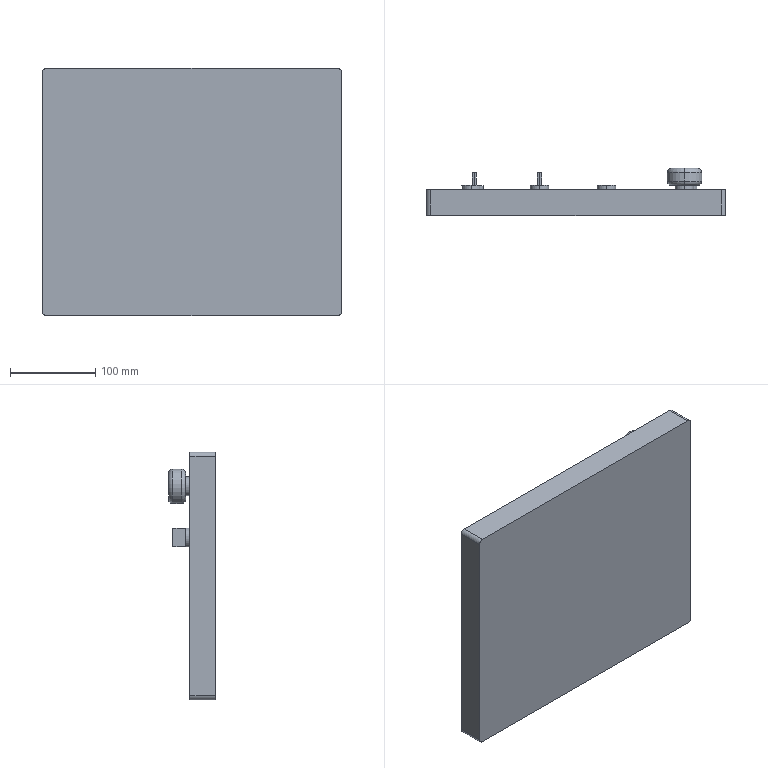Part | STEP file | Part 12 | 1 solid | 69 faces | box 350 x 55 x 290 mm | volume 3054092 mm3 | plane 33 | cylinder 32 | torus 4 | commonest cylinder face diameters 22 x16 19.283 x10 10 x4 40.309 x2